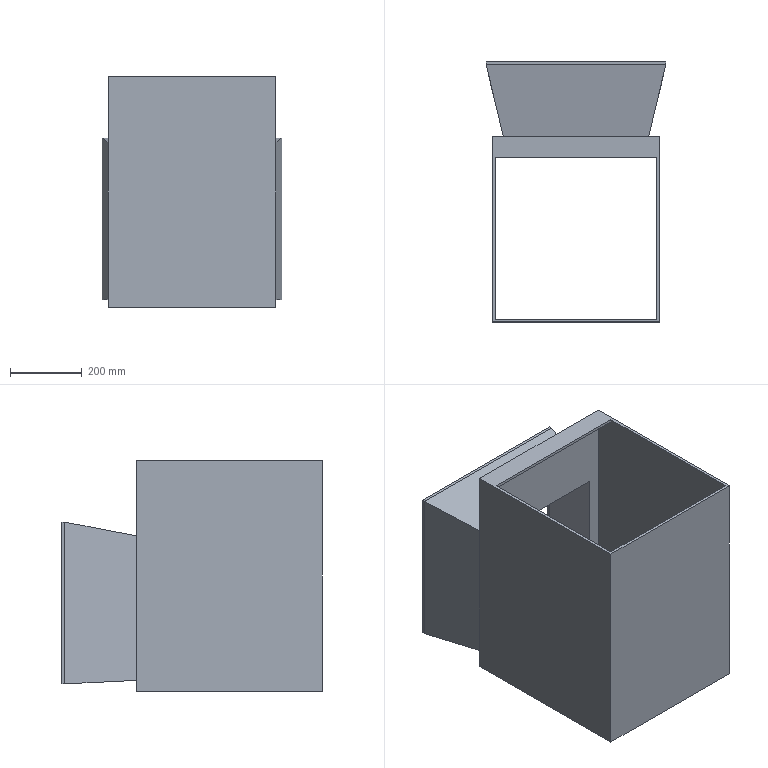Part | SolidWorks | features ICE 5, Blend 1, Extrusion 1, Shell 1 | 1 solid | 31 faces | box 500 x 724 x 640 mm | volume 11993841 mm3 | plane 31
STEP:
#1=CARTESIAN_POINT('',(191.772,250.,421.853));
#2=VERTEX_POINT('',#1);
#3=CARTESIAN_POINT('',(191.772,250.,38.009));
#4=VERTEX_POINT('',#3);
#5=CARTESIAN_POINT('',(191.772,250.,0.));
#6=DIRECTION('',(0.,0.,-1.));
#7=VECTOR('',#6,1000.);
#8=LINE('',#5,#7);
#9=EDGE_CURVE('',#2,#4,#8,.T.);
#10=ORIENTED_EDGE('',*,*,#9,.T.);
#11=CARTESIAN_POINT('',(-191.772,250.,38.009));
#12=VERTEX_POINT('',#11);
#13=CARTESIAN_POINT('',(0.,250.,38.009));
#14=DIRECTION('',(-1.,0.,0.));
#15=VECTOR('',#14,1000.);
#16=LINE('',#13,#15);
#17=EDGE_CURVE('',#4,#12,#16,.T.);
#18=ORIENTED_EDGE('',*,*,#17,.T.);
#19=CARTESIAN_POINT('',(-191.772,250.,421.853));
#20=VERTEX_POINT('',#19);
#21=CARTESIAN_POINT('',(-191.772,250.,0.));
#22=DIRECTION('',(0.,0.,1.));
#23=VECTOR('',#22,1000.);
#24=LINE('',#21,#23);
#25=EDGE_CURVE('',#12,#20,#24,.T.);
#26=ORIENTED_EDGE('',*,*,#25,.T.);
#27=CARTESIAN_POINT('',(0.,250.,421.853));
#28=DIRECTION('',(1.,0.,0.));
#29=VECTOR('',#28,1000.);
#30=LINE('',#27,#29);
#31=EDGE_CURVE('',#20,#2,#30,.T.);
#32=ORIENTED_EDGE('',*,*,#31,.T.);
#33=EDGE_LOOP('',(#10,#18,#26,#32));
#34=FACE_BOUND('',#33,.T.);
#35=CARTESIAN_POINT('',(-225.,250.,632.));
#36=VERTEX_POINT('',#35);
#37=CARTESIAN_POINT('',(225.,250.,632.));
#38=VERTEX_POINT('',#37);
#39=CARTESIAN_POINT('',(-233.,250.,632.));
#40=DIRECTION('',(1.,0.,0.));
#41=VECTOR('',#40,1000.);
#42=LINE('',#39,#41);
#43=EDGE_CURVE('',#36,#38,#42,.T.);
#44=ORIENTED_EDGE('',*,*,#43,.F.);
#45=CARTESIAN_POINT('',(-225.,250.,8.));
#46=VERTEX_POINT('',#45);
#47=CARTESIAN_POINT('',(-225.,250.,640.));
#48=DIRECTION('',(0.,0.,-1.));
#49=VECTOR('',#48,1000.);
#50=LINE('',#47,#49);
#51=EDGE_CURVE('',#36,#46,#50,.T.);
#52=ORIENTED_EDGE('',*,*,#51,.T.);
#53=CARTESIAN_POINT('',(225.,250.,8.));
#54=VERTEX_POINT('',#53);
#55=CARTESIAN_POINT('',(-233.,250.,8.));
#56=DIRECTION('',(-1.,0.,0.));
#57=VECTOR('',#56,1000.);
#58=LINE('',#55,#57);
#59=EDGE_CURVE('',#54,#46,#58,.T.);
#60=ORIENTED_EDGE('',*,*,#59,.F.);
#61=CARTESIAN_POINT('',(225.,250.,640.));
#62=DIRECTION('',(0.,0.,-1.));
#63=VECTOR('',#62,1000.);
#64=LINE('',#61,#63);
#65=EDGE_CURVE('',#38,#54,#64,.T.);
#66=ORIENTED_EDGE('',*,*,#65,.F.);
#67=EDGE_LOOP('',(#44,#52,#60,#66));
#68=FACE_OUTER_BOUND('',#67,.T.);
#69=CARTESIAN_POINT('',(0.,250.,0.));
#70=DIRECTION('',(0.,1.,0.));
#71=DIRECTION('',(0.,0.,1.));
#72=AXIS2_PLACEMENT_3D('',#69,#70,#71);
#73=PLANE('',#72);
#74=ADVANCED_FACE('',(#34,#68),#73,.F.);
#75=CARTESIAN_POINT('',(225.,200.,632.));
#76=VERTEX_POINT('',#75);
#77=CARTESIAN_POINT('',(225.,200.,640.));
#78=VERTEX_POINT('',#77);
#79=CARTESIAN_POINT('',(225.,200.,640.));
#80=DIRECTION('',(0.,0.,1.));
#81=VECTOR('',#80,1000.);
#82=LINE('',#79,#81);
#83=EDGE_CURVE('',#76,#78,#82,.T.);
#84=ORIENTED_EDGE('',*,*,#83,.F.);
#85=CARTESIAN_POINT('',(225.,250.,632.));
#86=DIRECTION('',(0.,1.,0.));
#87=VECTOR('',#86,1000.);
#88=LINE('',#85,#87);
#89=EDGE_CURVE('',#76,#38,#88,.T.);
#90=ORIENTED_EDGE('',*,*,#89,.T.);
#91=ORIENTED_EDGE('',*,*,#65,.T.);
#92=CARTESIAN_POINT('',(225.,200.,8.));
#93=VERTEX_POINT('',#92);
#94=CARTESIAN_POINT('',(225.,250.,8.));
#95=DIRECTION('',(0.,-1.,0.));
#96=VECTOR('',#95,1000.);
#97=LINE('',#94,#96);
#98=EDGE_CURVE('',#54,#93,#97,.T.);
#99=ORIENTED_EDGE('',*,*,#98,.T.);
#100=CARTESIAN_POINT('',(225.,200.,0.));
#101=VERTEX_POINT('',#100);
#102=CARTESIAN_POINT('',(225.,200.,640.));
#103=DIRECTION('',(0.,0.,-1.));
#104=VECTOR('',#103,1000.);
#105=LINE('',#102,#104);
#106=EDGE_CURVE('',#93,#101,#105,.T.);
#107=ORIENTED_EDGE('',*,*,#106,.T.);
#108=CARTESIAN_POINT('',(225.,-250.,0.));
#109=VERTEX_POINT('',#108);
#110=CARTESIAN_POINT('',(225.,250.,0.));
#111=DIRECTION('',(0.,1.,0.));
#112=VECTOR('',#111,1000.);
#113=LINE('',#110,#112);
#114=EDGE_CURVE('',#109,#101,#113,.T.);
#115=ORIENTED_EDGE('',*,*,#114,.F.);
#116=CARTESIAN_POINT('',(225.,-250.,640.));
#117=VERTEX_POINT('',#116);
#118=CARTESIAN_POINT('',(225.,-250.,640.));
#119=DIRECTION('',(0.,0.,-1.));
#120=VECTOR('',#119,1000.);
#121=LINE('',#118,#120);
#122=EDGE_CURVE('',#117,#109,#121,.T.);
#123=ORIENTED_EDGE('',*,*,#122,.F.);
#124=CARTESIAN_POINT('',(225.,250.,640.));
#125=DIRECTION('',(0.,1.,0.));
#126=VECTOR('',#125,1000.);
#127=LINE('',#124,#126);
#128=EDGE_CURVE('',#117,#78,#127,.T.);
#129=ORIENTED_EDGE('',*,*,#128,.T.);
#130=EDGE_LOOP('',(#84,#90,#91,#99,#107,#115,#123,#129));
#131=FACE_OUTER_BOUND('',#130,.T.);
#132=CARTESIAN_POINT('',(225.,250.,640.));
#133=DIRECTION('',(-1.,0.,0.));
#134=DIRECTION('',(0.,-1.,0.));
#135=AXIS2_PLACEMENT_3D('',#132,#133,#134);
#136=PLANE('',#135);
#137=ADVANCED_FACE('',(#131),#136,.T.);
#138=ORIENTED_EDGE('',*,*,#51,.F.);
#139=CARTESIAN_POINT('',(-225.,200.,632.));
#140=VERTEX_POINT('',#139);
#141=CARTESIAN_POINT('',(-225.,250.,632.));
#142=DIRECTION('',(0.,-1.,0.));
#143=VECTOR('',#142,1000.);
#144=LINE('',#141,#143);
#145=EDGE_CURVE('',#36,#140,#144,.T.);
#146=ORIENTED_EDGE('',*,*,#145,.T.);
#147=CARTESIAN_POINT('',(-225.,200.,640.));
#148=VERTEX_POINT('',#147);
#149=CARTESIAN_POINT('',(-225.,200.,640.));
#150=DIRECTION('',(0.,0.,-1.));
#151=VECTOR('',#150,1000.);
#152=LINE('',#149,#151);
#153=EDGE_CURVE('',#148,#140,#152,.T.);
#154=ORIENTED_EDGE('',*,*,#153,.F.);
#155=CARTESIAN_POINT('',(-225.,-250.,640.));
#156=VERTEX_POINT('',#155);
#157=CARTESIAN_POINT('',(-225.,250.,640.));
#158=DIRECTION('',(0.,-1.,0.));
#159=VECTOR('',#158,1000.);
#160=LINE('',#157,#159);
#161=EDGE_CURVE('',#148,#156,#160,.T.);
#162=ORIENTED_EDGE('',*,*,#161,.T.);
#163=CARTESIAN_POINT('',(-225.,-250.,0.));
#164=VERTEX_POINT('',#163);
#165=CARTESIAN_POINT('',(-225.,-250.,640.));
#166=DIRECTION('',(0.,0.,-1.));
#167=VECTOR('',#166,1000.);
#168=LINE('',#165,#167);
#169=EDGE_CURVE('',#156,#164,#168,.T.);
#170=ORIENTED_EDGE('',*,*,#169,.T.);
#171=CARTESIAN_POINT('',(-225.,200.,0.));
#172=VERTEX_POINT('',#171);
#173=CARTESIAN_POINT('',(-225.,250.,0.));
#174=DIRECTION('',(0.,-1.,0.));
#175=VECTOR('',#174,1000.);
#176=LINE('',#173,#175);
#177=EDGE_CURVE('',#172,#164,#176,.T.);
#178=ORIENTED_EDGE('',*,*,#177,.F.);
#179=CARTESIAN_POINT('',(-225.,200.,8.));
#180=VERTEX_POINT('',#179);
#181=CARTESIAN_POINT('',(-225.,200.,640.));
#182=DIRECTION('',(0.,0.,1.));
#183=VECTOR('',#182,1000.);
#184=LINE('',#181,#183);
#185=EDGE_CURVE('',#172,#180,#184,.T.);
#186=ORIENTED_EDGE('',*,*,#185,.T.);
#187=CARTESIAN_POINT('',(-225.,250.,8.));
#188=DIRECTION('',(0.,1.,0.));
#189=VECTOR('',#188,1000.);
#190=LINE('',#187,#189);
#191=EDGE_CURVE('',#180,#46,#190,.T.);
#192=ORIENTED_EDGE('',*,*,#191,.T.);
#193=EDGE_LOOP('',(#138,#146,#154,#162,#170,#178,#186,#192));
#194=FACE_OUTER_BOUND('',#193,.T.);
#195=CARTESIAN_POINT('',(-225.,250.,640.));
#196=DIRECTION('',(1.,0.,0.));
#197=DIRECTION('',(0.,1.,0.));
#198=AXIS2_PLACEMENT_3D('',#195,#196,#197);
#199=PLANE('',#198);
#200=ADVANCED_FACE('',(#194),#199,.T.);
#201=CARTESIAN_POINT('',(-250.,458.,470.));
#202=VERTEX_POINT('',#201);
#203=CARTESIAN_POINT('',(-201.923,258.,431.538));
#204=VERTEX_POINT('',#203);
#205=CARTESIAN_POINT('',(-250.,458.,470.));
#206=DIRECTION('',(0.2297,-0.9557,-0.1838));
#207=VECTOR('',#206,1000.);
#208=LINE('',#205,#207);
#209=EDGE_CURVE('',#202,#204,#208,.T.);
#210=ORIENTED_EDGE('',*,*,#209,.T.);
#211=CARTESIAN_POINT('',(201.923,258.,431.538));
#212=VERTEX_POINT('',#211);
#213=CARTESIAN_POINT('',(0.,258.,431.538));
#214=DIRECTION('',(1.,0.,0.));
#215=VECTOR('',#214,1000.);
#216=LINE('',#213,#215);
#217=EDGE_CURVE('',#204,#212,#216,.T.);
#218=ORIENTED_EDGE('',*,*,#217,.T.);
#219=CARTESIAN_POINT('',(250.,458.,470.));
#220=VERTEX_POINT('',#219);
#221=CARTESIAN_POINT('',(250.,458.,470.));
#222=DIRECTION('',(-0.2297,-0.9557,-0.1838));
#223=VECTOR('',#222,1000.);
#224=LINE('',#221,#223);
#225=EDGE_CURVE('',#220,#212,#224,.T.);
#226=ORIENTED_EDGE('',*,*,#225,.F.);
#227=CARTESIAN_POINT('',(-250.,458.,470.));
#228=DIRECTION('',(1.,0.,0.));
#229=VECTOR('',#228,1000.);
#230=LINE('',#227,#229);
#231=EDGE_CURVE('',#202,#220,#230,.T.);
#232=ORIENTED_EDGE('',*,*,#231,.F.);
#233=EDGE_LOOP('',(#210,#218,#226,#232));
#234=FACE_OUTER_BOUND('',#233,.T.);
#235=CARTESIAN_POINT('',(0.,-70.827,368.302));
#236=DIRECTION('',(0.,-0.1888,0.982));
#237=DIRECTION('',(0.,-0.982,-0.1888));
#238=AXIS2_PLACEMENT_3D('',#235,#236,#237);
#239=PLANE('',#238);
#240=ADVANCED_FACE('',(#234),#239,.T.);
#241=ORIENTED_EDGE('',*,*,#225,.T.);
#242=CARTESIAN_POINT('',(201.923,258.,29.615));
#243=VERTEX_POINT('',#242);
#244=CARTESIAN_POINT('',(201.923,258.,0.));
#245=DIRECTION('',(0.,0.,-1.));
#246=VECTOR('',#245,1000.);
#247=LINE('',#244,#246);
#248=EDGE_CURVE('',#212,#243,#247,.T.);
#249=ORIENTED_EDGE('',*,*,#248,.T.);
#250=CARTESIAN_POINT('',(250.,458.,20.));
#251=VERTEX_POINT('',#250);
#252=CARTESIAN_POINT('',(250.,458.,20.));
#253=DIRECTION('',(-0.2335,-0.9712,0.04669));
#254=VECTOR('',#253,1000.);
#255=LINE('',#252,#254);
#256=EDGE_CURVE('',#251,#243,#255,.T.);
#257=ORIENTED_EDGE('',*,*,#256,.F.);
#258=CARTESIAN_POINT('',(250.,458.,20.));
#259=DIRECTION('',(0.,0.,-1.));
#260=VECTOR('',#259,1000.);
#261=LINE('',#258,#260);
#262=EDGE_CURVE('',#220,#251,#261,.T.);
#263=ORIENTED_EDGE('',*,*,#262,.F.);
#264=EDGE_LOOP('',(#241,#249,#257,#263));
#265=FACE_OUTER_BOUND('',#264,.T.);
#266=CARTESIAN_POINT('',(132.261,-31.794,0.));
#267=DIRECTION('',(0.9723,-0.2337,0.));
#268=DIRECTION('',(0.2337,0.9723,0.));
#269=AXIS2_PLACEMENT_3D('',#266,#267,#268);
#270=PLANE('',#269);
#271=ADVANCED_FACE('',(#265),#270,.T.);
#272=ORIENTED_EDGE('',*,*,#256,.T.);
#273=CARTESIAN_POINT('',(-201.923,258.,29.615));
#274=VERTEX_POINT('',#273);
#275=CARTESIAN_POINT('',(0.,258.,29.615));
#276=DIRECTION('',(-1.,0.,0.));
#277=VECTOR('',#276,1000.);
#278=LINE('',#275,#277);
#279=EDGE_CURVE('',#243,#274,#278,.T.);
#280=ORIENTED_EDGE('',*,*,#279,.T.);
#281=CARTESIAN_POINT('',(-250.,458.,20.));
#282=VERTEX_POINT('',#281);
#283=CARTESIAN_POINT('',(-250.,458.,20.));
#284=DIRECTION('',(0.2335,-0.9712,0.04669));
#285=VECTOR('',#284,1000.);
#286=LINE('',#283,#285);
#287=EDGE_CURVE('',#282,#274,#286,.T.);
#288=ORIENTED_EDGE('',*,*,#287,.F.);
#289=CARTESIAN_POINT('',(-250.,458.,20.));
#290=DIRECTION('',(-1.,0.,0.));
#291=VECTOR('',#290,1000.);
#292=LINE('',#289,#291);
#293=EDGE_CURVE('',#251,#282,#292,.T.);
#294=ORIENTED_EDGE('',*,*,#293,.F.);
#295=EDGE_LOOP('',(#272,#280,#288,#294));
#296=FACE_OUTER_BOUND('',#295,.T.);
#297=CARTESIAN_POINT('',(0.,2.015,41.922));
#298=DIRECTION('',(0.,-0.04802,-0.9988));
#299=DIRECTION('',(0.,0.9988,-0.04802));
#300=AXIS2_PLACEMENT_3D('',#297,#298,#299);
#301=PLANE('',#300);
#302=ADVANCED_FACE('',(#296),#301,.T.);
#303=ORIENTED_EDGE('',*,*,#287,.T.);
#304=CARTESIAN_POINT('',(-201.923,258.,0.));
#305=DIRECTION('',(0.,0.,1.));
#306=VECTOR('',#305,1000.);
#307=LINE('',#304,#306);
#308=EDGE_CURVE('',#274,#204,#307,.T.);
#309=ORIENTED_EDGE('',*,*,#308,.T.);
#310=ORIENTED_EDGE('',*,*,#209,.F.);
#311=CARTESIAN_POINT('',(-250.,458.,20.));
#312=DIRECTION('',(0.,0.,1.));
#313=VECTOR('',#312,1000.);
#314=LINE('',#311,#313);
#315=EDGE_CURVE('',#282,#202,#314,.T.);
#316=ORIENTED_EDGE('',*,*,#315,.F.);
#317=EDGE_LOOP('',(#303,#309,#310,#316));
#318=FACE_OUTER_BOUND('',#317,.T.);
#319=CARTESIAN_POINT('',(-132.261,-31.794,0.));
#320=DIRECTION('',(-0.9723,-0.2337,0.));
#321=DIRECTION('',(0.2337,-0.9723,0.));
#322=AXIS2_PLACEMENT_3D('',#319,#320,#321);
#323=PLANE('',#322);
#324=ADVANCED_FACE('',(#318),#323,.T.);
#325=ORIENTED_EDGE('',*,*,#262,.T.);
#326=CARTESIAN_POINT('',(250.,466.,20.));
#327=VERTEX_POINT('',#326);
#328=CARTESIAN_POINT('',(250.,466.,20.));
#329=DIRECTION('',(0.,-1.,0.));
#330=VECTOR('',#329,1000.);
#331=LINE('',#328,#330);
#332=EDGE_CURVE('',#327,#251,#331,.T.);
#333=ORIENTED_EDGE('',*,*,#332,.F.);
#334=CARTESIAN_POINT('',(250.,466.,470.));
#335=VERTEX_POINT('',#334);
#336=CARTESIAN_POINT('',(250.,466.,20.));
#337=DIRECTION('',(0.,0.,-1.));
#338=VECTOR('',#337,1000.);
#339=LINE('',#336,#338);
#340=EDGE_CURVE('',#335,#327,#339,.T.);
#341=ORIENTED_EDGE('',*,*,#340,.F.);
#342=CARTESIAN_POINT('',(250.,466.,470.));
#343=DIRECTION('',(0.,-1.,0.));
#344=VECTOR('',#343,1000.);
#345=LINE('',#342,#344);
#346=EDGE_CURVE('',#335,#220,#345,.T.);
#347=ORIENTED_EDGE('',*,*,#346,.T.);
#348=EDGE_LOOP('',(#325,#333,#341,#347));
#349=FACE_OUTER_BOUND('',#348,.T.);
#350=CARTESIAN_POINT('',(250.,466.,20.));
#351=DIRECTION('',(-1.,0.,0.));
#352=DIRECTION('',(0.,0.,1.));
#353=AXIS2_PLACEMENT_3D('',#350,#351,#352);
#354=PLANE('',#353);
#355=ADVANCED_FACE('',(#349),#354,.F.);
#356=ORIENTED_EDGE('',*,*,#293,.T.);
#357=CARTESIAN_POINT('',(-250.,466.,20.));
#358=VERTEX_POINT('',#357);
#359=CARTESIAN_POINT('',(-250.,466.,20.));
#360=DIRECTION('',(0.,-1.,0.));
#361=VECTOR('',#360,1000.);
#362=LINE('',#359,#361);
#363=EDGE_CURVE('',#358,#282,#362,.T.);
#364=ORIENTED_EDGE('',*,*,#363,.F.);
#365=CARTESIAN_POINT('',(-250.,466.,20.));
#366=DIRECTION('',(-1.,0.,0.));
#367=VECTOR('',#366,1000.);
#368=LINE('',#365,#367);
#369=EDGE_CURVE('',#327,#358,#368,.T.);
#370=ORIENTED_EDGE('',*,*,#369,.F.);
#371=ORIENTED_EDGE('',*,*,#332,.T.);
#372=EDGE_LOOP('',(#356,#364,#370,#371));
#373=FACE_OUTER_BOUND('',#372,.T.);
#374=CARTESIAN_POINT('',(-250.,466.,20.));
#375=DIRECTION('',(0.,0.,1.));
#376=DIRECTION('',(1.,0.,0.));
#377=AXIS2_PLACEMENT_3D('',#374,#375,#376);
#378=PLANE('',#377);
#379=ADVANCED_FACE('',(#373),#378,.F.);
#380=ORIENTED_EDGE('',*,*,#315,.T.);
#381=CARTESIAN_POINT('',(-250.,466.,470.));
#382=VERTEX_POINT('',#381);
#383=CARTESIAN_POINT('',(-250.,466.,470.));
#384=DIRECTION('',(0.,-1.,0.));
#385=VECTOR('',#384,1000.);
#386=LINE('',#383,#385);
#387=EDGE_CURVE('',#382,#202,#386,.T.);
#388=ORIENTED_EDGE('',*,*,#387,.F.);
#389=CARTESIAN_POINT('',(-250.,466.,20.));
#390=DIRECTION('',(0.,0.,1.));
#391=VECTOR('',#390,1000.);
#392=LINE('',#389,#391);
#393=EDGE_CURVE('',#358,#382,#392,.T.);
#394=ORIENTED_EDGE('',*,*,#393,.F.);
#395=ORIENTED_EDGE('',*,*,#363,.T.);
#396=EDGE_LOOP('',(#380,#388,#394,#395));
#397=FACE_OUTER_BOUND('',#396,.T.);
#398=CARTESIAN_POINT('',(-250.,466.,20.));
#399=DIRECTION('',(1.,0.,0.));
#400=DIRECTION('',(0.,0.,-1.));
#401=AXIS2_PLACEMENT_3D('',#398,#399,#400);
#402=PLANE('',#401);
#403=ADVANCED_FACE('',(#397),#402,.F.);
#404=ORIENTED_EDGE('',*,*,#231,.T.);
#405=ORIENTED_EDGE('',*,*,#346,.F.);
#406=CARTESIAN_POINT('',(-250.,466.,470.));
#407=DIRECTION('',(1.,0.,0.));
#408=VECTOR('',#407,1000.);
#409=LINE('',#406,#408);
#410=EDGE_CURVE('',#382,#335,#409,.T.);
#411=ORIENTED_EDGE('',*,*,#410,.F.);
#412=ORIENTED_EDGE('',*,*,#387,.T.);
#413=EDGE_LOOP('',(#404,#405,#411,#412));
#414=FACE_OUTER_BOUND('',#413,.T.);
#415=CARTESIAN_POINT('',(-250.,466.,470.));
#416=DIRECTION('',(0.,0.,-1.));
#417=DIRECTION('',(-1.,0.,0.));
#418=AXIS2_PLACEMENT_3D('',#415,#416,#417);
#419=PLANE('',#418);
#420=ADVANCED_FACE('',(#414),#419,.F.);
#421=CARTESIAN_POINT('',(242.,466.,462.));
#422=VERTEX_POINT('',#421);
#423=CARTESIAN_POINT('',(242.,466.,28.));
#424=VERTEX_POINT('',#423);
#425=CARTESIAN_POINT('',(242.,466.,20.));
#426=DIRECTION('',(0.,0.,-1.));
#427=VECTOR('',#426,1000.);
#428=LINE('',#425,#427);
#429=EDGE_CURVE('',#422,#424,#428,.T.);
#430=ORIENTED_EDGE('',*,*,#429,.F.);
#431=CARTESIAN_POINT('',(-242.,466.,462.));
#432=VERTEX_POINT('',#431);
#433=CARTESIAN_POINT('',(-250.,466.,462.));
#434=DIRECTION('',(1.,0.,0.));
#435=VECTOR('',#434,1000.);
#436=LINE('',#433,#435);
#437=EDGE_CURVE('',#432,#422,#436,.T.);
#438=ORIENTED_EDGE('',*,*,#437,.F.);
#439=CARTESIAN_POINT('',(-242.,466.,28.));
#440=VERTEX_POINT('',#439);
#441=CARTESIAN_POINT('',(-242.,466.,20.));
#442=DIRECTION('',(0.,0.,1.));
#443=VECTOR('',#442,1000.);
#444=LINE('',#441,#443);
#445=EDGE_CURVE('',#440,#432,#444,.T.);
#446=ORIENTED_EDGE('',*,*,#445,.F.);
#447=CARTESIAN_POINT('',(-250.,466.,28.));
#448=DIRECTION('',(-1.,0.,0.));
#449=VECTOR('',#448,1000.);
#450=LINE('',#447,#449);
#451=EDGE_CURVE('',#424,#440,#450,.T.);
#452=ORIENTED_EDGE('',*,*,#451,.F.);
#453=EDGE_LOOP('',(#430,#438,#446,#452));
#454=FACE_BOUND('',#453,.T.);
#455=ORIENTED_EDGE('',*,*,#340,.T.);
#456=ORIENTED_EDGE('',*,*,#369,.T.);
#457=ORIENTED_EDGE('',*,*,#393,.T.);
#458=ORIENTED_EDGE('',*,*,#410,.T.);
#459=EDGE_LOOP('',(#455,#456,#457,#458));
#460=FACE_OUTER_BOUND('',#459,.T.);
#461=CARTESIAN_POINT('',(0.,466.,0.));
#462=DIRECTION('',(0.,1.,0.));
#463=DIRECTION('',(0.,0.,1.));
#464=AXIS2_PLACEMENT_3D('',#461,#462,#463);
#465=PLANE('',#464);
#466=ADVANCED_FACE('',(#454,#460),#465,.T.);
#467=ORIENTED_EDGE('',*,*,#161,.F.);
#468=CARTESIAN_POINT('',(-233.,200.,640.));
#469=DIRECTION('',(-1.,0.,0.));
#470=VECTOR('',#469,1000.);
#471=LINE('',#468,#470);
#472=EDGE_CURVE('',#78,#148,#471,.T.);
#473=ORIENTED_EDGE('',*,*,#472,.F.);
#474=ORIENTED_EDGE('',*,*,#128,.F.);
#475=CARTESIAN_POINT('',(-225.,-250.,640.));
#476=DIRECTION('',(1.,0.,0.));
#477=VECTOR('',#476,1000.);
#478=LINE('',#475,#477);
#479=EDGE_CURVE('',#156,#117,#478,.T.);
#480=ORIENTED_EDGE('',*,*,#479,.F.);
#481=EDGE_LOOP('',(#467,#473,#474,#480));
#482=FACE_BOUND('',#481,.T.);
#483=CARTESIAN_POINT('',(-233.,258.,640.));
#484=VERTEX_POINT('',#483);
#485=CARTESIAN_POINT('',(-233.,-258.,640.));
#486=VERTEX_POINT('',#485);
#487=CARTESIAN_POINT('',(-233.,258.,640.));
#488=DIRECTION('',(0.,-1.,0.));
#489=VECTOR('',#488,1000.);
#490=LINE('',#487,#489);
#491=EDGE_CURVE('',#484,#486,#490,.T.);
#492=ORIENTED_EDGE('',*,*,#491,.T.);
#493=CARTESIAN_POINT('',(233.,-258.,640.));
#494=VERTEX_POINT('',#493);
#495=CARTESIAN_POINT('',(-233.,-258.,640.));
#496=DIRECTION('',(1.,0.,0.));
#497=VECTOR('',#496,1000.);
#498=LINE('',#495,#497);
#499=EDGE_CURVE('',#486,#494,#498,.T.);
#500=ORIENTED_EDGE('',*,*,#499,.T.);
#501=CARTESIAN_POINT('',(233.,258.,640.));
#502=VERTEX_POINT('',#501);
#503=CARTESIAN_POINT('',(233.,258.,640.));
#504=DIRECTION('',(0.,1.,0.));
#505=VECTOR('',#504,1000.);
#506=LINE('',#503,#505);
#507=EDGE_CURVE('',#494,#502,#506,.T.);
#508=ORIENTED_EDGE('',*,*,#507,.T.);
#509=CARTESIAN_POINT('',(-233.,258.,640.));
#510=DIRECTION('',(-1.,0.,0.));
#511=VECTOR('',#510,1000.);
#512=LINE('',#509,#511);
#513=EDGE_CURVE('',#502,#484,#512,.T.);
#514=ORIENTED_EDGE('',*,*,#513,.T.);
#515=EDGE_LOOP('',(#492,#500,#508,#514));
#516=FACE_OUTER_BOUND('',#515,.T.);
#517=CARTESIAN_POINT('',(0.,0.,640.));
#518=DIRECTION('',(0.,0.,1.));
#519=DIRECTION('',(1.,0.,0.));
#520=AXIS2_PLACEMENT_3D('',#517,#518,#519);
#521=PLANE('',#520);
#522=ADVANCED_FACE('',(#482,#516),#521,.T.);
#523=ORIENTED_EDGE('',*,*,#114,.T.);
#524=CARTESIAN_POINT('',(-233.,200.,0.));
#525=DIRECTION('',(1.,0.,0.));
#526=VECTOR('',#525,1000.);
#527=LINE('',#524,#526);
#528=EDGE_CURVE('',#172,#101,#527,.T.);
#529=ORIENTED_EDGE('',*,*,#528,.F.);
#530=ORIENTED_EDGE('',*,*,#177,.T.);
#531=CARTESIAN_POINT('',(-225.,-250.,0.));
#532=DIRECTION('',(1.,0.,0.));
#533=VECTOR('',#532,1000.);
#534=LINE('',#531,#533);
#535=EDGE_CURVE('',#164,#109,#534,.T.);
#536=ORIENTED_EDGE('',*,*,#535,.T.);
#537=EDGE_LOOP('',(#523,#529,#530,#536));
#538=FACE_BOUND('',#537,.T.);
#539=CARTESIAN_POINT('',(233.,258.,0.));
#540=VERTEX_POINT('',#539);
#541=CARTESIAN_POINT('',(-233.,258.,0.));
#542=VERTEX_POINT('',#541);
#543=CARTESIAN_POINT('',(-233.,258.,0.));
#544=DIRECTION('',(-1.,0.,0.));
#545=VECTOR('',#544,1000.);
#546=LINE('',#543,#545);
#547=EDGE_CURVE('',#540,#542,#546,.T.);
#548=ORIENTED_EDGE('',*,*,#547,.F.);
#549=CARTESIAN_POINT('',(233.,-258.,0.));
#550=VERTEX_POINT('',#549);
#551=CARTESIAN_POINT('',(233.,258.,0.));
#552=DIRECTION('',(0.,1.,0.));
#553=VECTOR('',#552,1000.);
#554=LINE('',#551,#553);
#555=EDGE_CURVE('',#550,#540,#554,.T.);
#556=ORIENTED_EDGE('',*,*,#555,.F.);
#557=CARTESIAN_POINT('',(-233.,-258.,0.));
#558=VERTEX_POINT('',#557);
#559=CARTESIAN_POINT('',(-233.,-258.,0.));
#560=DIRECTION('',(1.,0.,0.));
#561=VECTOR('',#560,1000.);
#562=LINE('',#559,#561);
#563=EDGE_CURVE('',#558,#550,#562,.T.);
#564=ORIENTED_EDGE('',*,*,#563,.F.);
#565=CARTESIAN_POINT('',(-233.,258.,0.));
#566=DIRECTION('',(0.,-1.,0.));
#567=VECTOR('',#566,1000.);
#568=LINE('',#565,#567);
#569=EDGE_CURVE('',#542,#558,#568,.T.);
#570=ORIENTED_EDGE('',*,*,#569,.F.);
#571=EDGE_LOOP('',(#548,#556,#564,#570));
#572=FACE_OUTER_BOUND('',#571,.T.);
#573=CARTESIAN_POINT('',(0.,0.,0.));
#574=DIRECTION('',(0.,0.,1.));
#575=DIRECTION('',(1.,0.,0.));
#576=AXIS2_PLACEMENT_3D('',#573,#574,#575);
#577=PLANE('',#576);
#578=ADVANCED_FACE('',(#538,#572),#577,.F.);
#579=CARTESIAN_POINT('',(233.,258.,640.));
#580=DIRECTION('',(0.,0.,-1.));
#581=VECTOR('',#580,1000.);
#582=LINE('',#579,#581);
#583=EDGE_CURVE('',#502,#540,#582,.T.);
#584=ORIENTED_EDGE('',*,*,#583,.F.);
#585=ORIENTED_EDGE('',*,*,#507,.F.);
#586=CARTESIAN_POINT('',(233.,-258.,640.));
#587=DIRECTION('',(0.,0.,-1.));
#588=VECTOR('',#587,1000.);
#589=LINE('',#586,#588);
#590=EDGE_CURVE('',#494,#550,#589,.T.);
#591=ORIENTED_EDGE('',*,*,#590,.T.);
#592=ORIENTED_EDGE('',*,*,#555,.T.);
#593=EDGE_LOOP('',(#584,#585,#591,#592));
#594=FACE_OUTER_BOUND('',#593,.T.);
#595=CARTESIAN_POINT('',(233.,258.,640.));
#596=DIRECTION('',(-1.,0.,0.));
#597=DIRECTION('',(0.,-1.,0.));
#598=AXIS2_PLACEMENT_3D('',#595,#596,#597);
#599=PLANE('',#598);
#600=ADVANCED_FACE('',(#594),#599,.F.);
#601=ORIENTED_EDGE('',*,*,#217,.F.);
#602=ORIENTED_EDGE('',*,*,#308,.F.);
#603=ORIENTED_EDGE('',*,*,#279,.F.);
#604=ORIENTED_EDGE('',*,*,#248,.F.);
#605=EDGE_LOOP('',(#601,#602,#603,#604));
#606=FACE_BOUND('',#605,.T.);
#607=ORIENTED_EDGE('',*,*,#547,.T.);
#608=CARTESIAN_POINT('',(-233.,258.,640.));
#609=DIRECTION('',(0.,0.,-1.));
#610=VECTOR('',#609,1000.);
#611=LINE('',#608,#610);
#612=EDGE_CURVE('',#484,#542,#611,.T.);
#613=ORIENTED_EDGE('',*,*,#612,.F.);
#614=ORIENTED_EDGE('',*,*,#513,.F.);
#615=ORIENTED_EDGE('',*,*,#583,.T.);
#616=EDGE_LOOP('',(#607,#613,#614,#615));
#617=FACE_OUTER_BOUND('',#616,.T.);
#618=CARTESIAN_POINT('',(-233.,258.,640.));
#619=DIRECTION('',(0.,-1.,0.));
#620=DIRECTION('',(0.,0.,-1.));
#621=AXIS2_PLACEMENT_3D('',#618,#619,#620);
#622=PLANE('',#621);
#623=ADVANCED_FACE('',(#606,#617),#622,.F.);
#624=ORIENTED_EDGE('',*,*,#569,.T.);
#625=CARTESIAN_POINT('',(-233.,-258.,640.));
#626=DIRECTION('',(0.,0.,-1.));
#627=VECTOR('',#626,1000.);
#628=LINE('',#625,#627);
#629=EDGE_CURVE('',#486,#558,#628,.T.);
#630=ORIENTED_EDGE('',*,*,#629,.F.);
#631=ORIENTED_EDGE('',*,*,#491,.F.);
#632=ORIENTED_EDGE('',*,*,#612,.T.);
#633=EDGE_LOOP('',(#624,#630,#631,#632));
#634=FACE_OUTER_BOUND('',#633,.T.);
#635=CARTESIAN_POINT('',(-233.,258.,640.));
#636=DIRECTION('',(1.,0.,0.));
#637=DIRECTION('',(0.,1.,0.));
#638=AXIS2_PLACEMENT_3D('',#635,#636,#637);
#639=PLANE('',#638);
#640=ADVANCED_FACE('',(#634),#639,.F.);
#641=ORIENTED_EDGE('',*,*,#563,.T.);
#642=ORIENTED_EDGE('',*,*,#590,.F.);
#643=ORIENTED_EDGE('',*,*,#499,.F.);
#644=ORIENTED_EDGE('',*,*,#629,.T.);
#645=EDGE_LOOP('',(#641,#642,#643,#644));
#646=FACE_OUTER_BOUND('',#645,.T.);
#647=CARTESIAN_POINT('',(-233.,-258.,640.));
#648=DIRECTION('',(0.,1.,0.));
#649=DIRECTION('',(0.,0.,1.));
#650=AXIS2_PLACEMENT_3D('',#647,#648,#649);
#651=PLANE('',#650);
#652=ADVANCED_FACE('',(#646),#651,.F.);
#653=ORIENTED_EDGE('',*,*,#535,.F.);
#654=ORIENTED_EDGE('',*,*,#169,.F.);
#655=ORIENTED_EDGE('',*,*,#479,.T.);
#656=ORIENTED_EDGE('',*,*,#122,.T.);
#657=EDGE_LOOP('',(#653,#654,#655,#656));
#658=FACE_OUTER_BOUND('',#657,.T.);
#659=CARTESIAN_POINT('',(-225.,-250.,640.));
#660=DIRECTION('',(0.,1.,0.));
#661=DIRECTION('',(0.,0.,1.));
#662=AXIS2_PLACEMENT_3D('',#659,#660,#661);
#663=PLANE('',#662);
#664=ADVANCED_FACE('',(#658),#663,.T.);
#665=CARTESIAN_POINT('',(241.955,458.762,462.));
#666=VERTEX_POINT('',#665);
#667=CARTESIAN_POINT('',(108.943,-94.571,355.59));
#668=DIRECTION('',(-0.2297,-0.9557,-0.1838));
#669=VECTOR('',#668,1000.);
#670=LINE('',#667,#669);
#671=EDGE_CURVE('',#666,#2,#670,.T.);
#672=ORIENTED_EDGE('',*,*,#671,.F.);
#673=CARTESIAN_POINT('',(242.,458.948,462.));
#674=VERTEX_POINT('',#673);
#675=CARTESIAN_POINT('',(124.483,-29.924,462.));
#676=DIRECTION('',(0.2337,0.9723,0.));
#677=VECTOR('',#676,1000.);
#678=LINE('',#675,#677);
#679=EDGE_CURVE('',#666,#674,#678,.T.);
#680=ORIENTED_EDGE('',*,*,#679,.T.);
#681=CARTESIAN_POINT('',(242.,458.948,28.));
#682=VERTEX_POINT('',#681);
#683=CARTESIAN_POINT('',(242.,458.948,0.));
#684=DIRECTION('',(0.,0.,-1.));
#685=VECTOR('',#684,1000.);
#686=LINE('',#683,#685);
#687=EDGE_CURVE('',#674,#682,#686,.T.);
#688=ORIENTED_EDGE('',*,*,#687,.T.);
#689=CARTESIAN_POINT('',(241.818,458.192,28.));
#690=VERTEX_POINT('',#689);
#691=CARTESIAN_POINT('',(216.726,353.806,28.));
#692=DIRECTION('',(0.2337,0.9723,0.));
#693=VECTOR('',#692,1000.);
#694=LINE('',#691,#693);
#695=EDGE_CURVE('',#690,#682,#694,.T.);
#696=ORIENTED_EDGE('',*,*,#695,.F.);
#697=CARTESIAN_POINT('',(125.044,-27.59,51.355));
#698=DIRECTION('',(-0.2335,-0.9712,0.04669));
#699=VECTOR('',#698,1000.);
#700=LINE('',#697,#699);
#701=EDGE_CURVE('',#690,#4,#700,.T.);
#702=ORIENTED_EDGE('',*,*,#701,.T.);
#703=ORIENTED_EDGE('',*,*,#9,.F.);
#704=EDGE_LOOP('',(#672,#680,#688,#696,#702,#703));
#705=FACE_OUTER_BOUND('',#704,.T.);
#706=CARTESIAN_POINT('',(124.483,-29.924,0.));
#707=DIRECTION('',(0.9723,-0.2337,0.));
#708=DIRECTION('',(0.2337,0.9723,0.));
#709=AXIS2_PLACEMENT_3D('',#706,#707,#708);
#710=PLANE('',#709);
#711=ADVANCED_FACE('',(#705),#710,.F.);
#712=ORIENTED_EDGE('',*,*,#701,.F.);
#713=CARTESIAN_POINT('',(-241.818,458.192,28.));
#714=VERTEX_POINT('',#713);
#715=CARTESIAN_POINT('',(0.,458.192,28.));
#716=DIRECTION('',(-1.,0.,0.));
#717=VECTOR('',#716,1000.);
#718=LINE('',#715,#717);
#719=EDGE_CURVE('',#690,#714,#718,.T.);
#720=ORIENTED_EDGE('',*,*,#719,.T.);
#721=CARTESIAN_POINT('',(-125.044,-27.59,51.355));
#722=DIRECTION('',(0.2335,-0.9712,0.04669));
#723=VECTOR('',#722,1000.);
#724=LINE('',#721,#723);
#725=EDGE_CURVE('',#714,#12,#724,.T.);
#726=ORIENTED_EDGE('',*,*,#725,.T.);
#727=ORIENTED_EDGE('',*,*,#17,.F.);
#728=EDGE_LOOP('',(#712,#720,#726,#727));
#729=FACE_OUTER_BOUND('',#728,.T.);
#730=CARTESIAN_POINT('',(0.,2.4,49.913));
#731=DIRECTION('',(0.,-0.04802,-0.9988));
#732=DIRECTION('',(0.,0.9988,-0.04802));
#733=AXIS2_PLACEMENT_3D('',#730,#731,#732);
#734=PLANE('',#733);
#735=ADVANCED_FACE('',(#729),#734,.F.);
#736=CARTESIAN_POINT('',(-241.955,458.762,462.));
#737=VERTEX_POINT('',#736);
#738=CARTESIAN_POINT('',(-108.943,-94.571,355.59));
#739=DIRECTION('',(0.2297,-0.9557,-0.1838));
#740=VECTOR('',#739,1000.);
#741=LINE('',#738,#740);
#742=EDGE_CURVE('',#737,#20,#741,.T.);
#743=ORIENTED_EDGE('',*,*,#742,.F.);
#744=CARTESIAN_POINT('',(0.,458.762,462.));
#745=DIRECTION('',(1.,0.,0.));
#746=VECTOR('',#745,1000.);
#747=LINE('',#744,#746);
#748=EDGE_CURVE('',#737,#666,#747,.T.);
#749=ORIENTED_EDGE('',*,*,#748,.T.);
#750=ORIENTED_EDGE('',*,*,#671,.T.);
#751=ORIENTED_EDGE('',*,*,#31,.F.);
#752=EDGE_LOOP('',(#743,#749,#750,#751));
#753=FACE_OUTER_BOUND('',#752,.T.);
#754=CARTESIAN_POINT('',(0.,-69.317,360.446));
#755=DIRECTION('',(0.,-0.1888,0.982));
#756=DIRECTION('',(0.,-0.982,-0.1888));
#757=AXIS2_PLACEMENT_3D('',#754,#755,#756);
#758=PLANE('',#757);
#759=ADVANCED_FACE('',(#753),#758,.F.);
#760=ORIENTED_EDGE('',*,*,#725,.F.);
#761=CARTESIAN_POINT('',(-242.,458.948,28.));
#762=VERTEX_POINT('',#761);
#763=CARTESIAN_POINT('',(-124.483,-29.924,28.));
#764=DIRECTION('',(-0.2337,0.9723,0.));
#765=VECTOR('',#764,1000.);
#766=LINE('',#763,#765);
#767=EDGE_CURVE('',#714,#762,#766,.T.);
#768=ORIENTED_EDGE('',*,*,#767,.T.);
#769=CARTESIAN_POINT('',(-242.,458.948,462.));
#770=VERTEX_POINT('',#769);
#771=CARTESIAN_POINT('',(-242.,458.948,0.));
#772=DIRECTION('',(0.,0.,1.));
#773=VECTOR('',#772,1000.);
#774=LINE('',#771,#773);
#775=EDGE_CURVE('',#762,#770,#774,.T.);
#776=ORIENTED_EDGE('',*,*,#775,.T.);
#777=CARTESIAN_POINT('',(-244.04,467.433,462.));
#778=DIRECTION('',(-0.2337,0.9723,0.));
#779=VECTOR('',#778,1000.);
#780=LINE('',#777,#779);
#781=EDGE_CURVE('',#737,#770,#780,.T.);
#782=ORIENTED_EDGE('',*,*,#781,.F.);
#783=ORIENTED_EDGE('',*,*,#742,.T.);
#784=ORIENTED_EDGE('',*,*,#25,.F.);
#785=EDGE_LOOP('',(#760,#768,#776,#782,#783,#784));
#786=FACE_OUTER_BOUND('',#785,.T.);
#787=CARTESIAN_POINT('',(-124.483,-29.924,0.));
#788=DIRECTION('',(-0.9723,-0.2337,0.));
#789=DIRECTION('',(0.2337,-0.9723,0.));
#790=AXIS2_PLACEMENT_3D('',#787,#788,#789);
#791=PLANE('',#790);
#792=ADVANCED_FACE('',(#786),#791,.F.);
#793=ORIENTED_EDGE('',*,*,#687,.F.);
#794=CARTESIAN_POINT('',(242.,466.,462.));
#795=DIRECTION('',(0.,-1.,0.));
#796=VECTOR('',#795,1000.);
#797=LINE('',#794,#796);
#798=EDGE_CURVE('',#422,#674,#797,.T.);
#799=ORIENTED_EDGE('',*,*,#798,.F.);
#800=ORIENTED_EDGE('',*,*,#429,.T.);
#801=CARTESIAN_POINT('',(242.,466.,28.));
#802=DIRECTION('',(0.,-1.,0.));
#803=VECTOR('',#802,1000.);
#804=LINE('',#801,#803);
#805=EDGE_CURVE('',#424,#682,#804,.T.);
#806=ORIENTED_EDGE('',*,*,#805,.T.);
#807=EDGE_LOOP('',(#793,#799,#800,#806));
#808=FACE_OUTER_BOUND('',#807,.T.);
#809=CARTESIAN_POINT('',(242.,466.,20.));
#810=DIRECTION('',(-1.,0.,0.));
#811=DIRECTION('',(0.,0.,1.));
#812=AXIS2_PLACEMENT_3D('',#809,#810,#811);
#813=PLANE('',#812);
#814=ADVANCED_FACE('',(#808),#813,.T.);
#815=ORIENTED_EDGE('',*,*,#719,.F.);
#816=ORIENTED_EDGE('',*,*,#695,.T.);
#817=ORIENTED_EDGE('',*,*,#805,.F.);
#818=ORIENTED_EDGE('',*,*,#451,.T.);
#819=CARTESIAN_POINT('',(-242.,466.,28.));
#820=DIRECTION('',(0.,-1.,0.));
#821=VECTOR('',#820,1000.);
#822=LINE('',#819,#821);
#823=EDGE_CURVE('',#440,#762,#822,.T.);
#824=ORIENTED_EDGE('',*,*,#823,.T.);
#825=ORIENTED_EDGE('',*,*,#767,.F.);
#826=EDGE_LOOP('',(#815,#816,#817,#818,#824,#825));
#827=FACE_OUTER_BOUND('',#826,.T.);
#828=CARTESIAN_POINT('',(-250.,466.,28.));
#829=DIRECTION('',(0.,0.,1.));
#830=DIRECTION('',(1.,0.,0.));
#831=AXIS2_PLACEMENT_3D('',#828,#829,#830);
#832=PLANE('',#831);
#833=ADVANCED_FACE('',(#827),#832,.T.);
#834=ORIENTED_EDGE('',*,*,#775,.F.);
#835=ORIENTED_EDGE('',*,*,#823,.F.);
#836=ORIENTED_EDGE('',*,*,#445,.T.);
#837=CARTESIAN_POINT('',(-242.,466.,462.));
#838=DIRECTION('',(0.,-1.,0.));
#839=VECTOR('',#838,1000.);
#840=LINE('',#837,#839);
#841=EDGE_CURVE('',#432,#770,#840,.T.);
#842=ORIENTED_EDGE('',*,*,#841,.T.);
#843=EDGE_LOOP('',(#834,#835,#836,#842));
#844=FACE_OUTER_BOUND('',#843,.T.);
#845=CARTESIAN_POINT('',(-242.,466.,20.));
#846=DIRECTION('',(1.,0.,0.));
#847=DIRECTION('',(0.,0.,-1.));
#848=AXIS2_PLACEMENT_3D('',#845,#846,#847);
#849=PLANE('',#848);
#850=ADVANCED_FACE('',(#844),#849,.T.);
#851=ORIENTED_EDGE('',*,*,#748,.F.);
#852=ORIENTED_EDGE('',*,*,#781,.T.);
#853=ORIENTED_EDGE('',*,*,#841,.F.);
#854=ORIENTED_EDGE('',*,*,#437,.T.);
#855=ORIENTED_EDGE('',*,*,#798,.T.);
#856=ORIENTED_EDGE('',*,*,#679,.F.);
#857=EDGE_LOOP('',(#851,#852,#853,#854,#855,#856));
#858=FACE_OUTER_BOUND('',#857,.T.);
#859=CARTESIAN_POINT('',(-250.,466.,462.));
#860=DIRECTION('',(0.,0.,-1.));
#861=DIRECTION('',(-1.,0.,0.));
#862=AXIS2_PLACEMENT_3D('',#859,#860,#861);
#863=PLANE('',#862);
#864=ADVANCED_FACE('',(#858),#863,.T.);
#865=ORIENTED_EDGE('',*,*,#98,.F.);
#866=ORIENTED_EDGE('',*,*,#59,.T.);
#867=ORIENTED_EDGE('',*,*,#191,.F.);
#868=CARTESIAN_POINT('',(-233.,200.,8.));
#869=DIRECTION('',(-1.,0.,0.));
#870=VECTOR('',#869,1000.);
#871=LINE('',#868,#870);
#872=EDGE_CURVE('',#93,#180,#871,.T.);
#873=ORIENTED_EDGE('',*,*,#872,.F.);
#874=EDGE_LOOP('',(#865,#866,#867,#873));
#875=FACE_OUTER_BOUND('',#874,.T.);
#876=CARTESIAN_POINT('',(-233.,200.,8.));
#877=DIRECTION('',(0.,0.,-1.));
#878=DIRECTION('',(-1.,0.,0.));
#879=AXIS2_PLACEMENT_3D('',#876,#877,#878);
#880=PLANE('',#879);
#881=ADVANCED_FACE('',(#875),#880,.F.);
#882=ORIENTED_EDGE('',*,*,#106,.F.);
#883=ORIENTED_EDGE('',*,*,#872,.T.);
#884=ORIENTED_EDGE('',*,*,#185,.F.);
#885=ORIENTED_EDGE('',*,*,#528,.T.);
#886=EDGE_LOOP('',(#882,#883,#884,#885));
#887=FACE_OUTER_BOUND('',#886,.T.);
#888=CARTESIAN_POINT('',(0.,200.,0.));
#889=DIRECTION('',(0.,1.,0.));
#890=DIRECTION('',(0.,0.,1.));
#891=AXIS2_PLACEMENT_3D('',#888,#889,#890);
#892=PLANE('',#891);
#893=ADVANCED_FACE('',(#887),#892,.F.);
#894=ORIENTED_EDGE('',*,*,#89,.F.);
#895=CARTESIAN_POINT('',(-233.,200.,632.));
#896=DIRECTION('',(1.,0.,0.));
#897=VECTOR('',#896,1000.);
#898=LINE('',#895,#897);
#899=EDGE_CURVE('',#140,#76,#898,.T.);
#900=ORIENTED_EDGE('',*,*,#899,.F.);
#901=ORIENTED_EDGE('',*,*,#145,.F.);
#902=ORIENTED_EDGE('',*,*,#43,.T.);
#903=EDGE_LOOP('',(#894,#900,#901,#902));
#904=FACE_OUTER_BOUND('',#903,.T.);
#905=CARTESIAN_POINT('',(-233.,200.,632.));
#906=DIRECTION('',(0.,0.,1.));
#907=DIRECTION('',(1.,0.,0.));
#908=AXIS2_PLACEMENT_3D('',#905,#906,#907);
#909=PLANE('',#908);
#910=ADVANCED_FACE('',(#904),#909,.F.);
#911=ORIENTED_EDGE('',*,*,#899,.T.);
#912=ORIENTED_EDGE('',*,*,#83,.T.);
#913=ORIENTED_EDGE('',*,*,#472,.T.);
#914=ORIENTED_EDGE('',*,*,#153,.T.);
#915=EDGE_LOOP('',(#911,#912,#913,#914));
#916=FACE_OUTER_BOUND('',#915,.T.);
#917=CARTESIAN_POINT('',(0.,200.,0.));
#918=DIRECTION('',(0.,-1.,0.));
#919=DIRECTION('',(0.,0.,-1.));
#920=AXIS2_PLACEMENT_3D('',#917,#918,#919);
#921=PLANE('',#920);
#922=ADVANCED_FACE('',(#916),#921,.T.);
#923=CLOSED_SHELL('',(#74,#137,#200,#240,#271,#302,#324,#355,#379,#403,#420,#466,#522,#578,#600,#623,#640,#652,#664,#711,#735,#759,#792,#814,#833,#850,#864,#881,#893,#910,#922));
#924=MANIFOLD_SOLID_BREP('',#923);
#925=CARTESIAN_POINT('',(0.,0.,0.));
#926=DIRECTION('',(0.,0.,1.));
#927=DIRECTION('',(1.,0.,0.));
#928=AXIS2_PLACEMENT_3D('',#925,#926,#927);
#929=(LENGTH_UNIT()NAMED_UNIT(*)SI_UNIT(.MILLI.,.METRE.));
#930=UNCERTAINTY_MEASURE_WITH_UNIT(LENGTH_MEASURE(0.00001),#929,'','');
#931=(NAMED_UNIT(*)PLANE_ANGLE_UNIT()SI_UNIT($,.RADIAN.));
#932=(NAMED_UNIT(*)SI_UNIT($,.STERADIAN.)SOLID_ANGLE_UNIT());
#933=(GEOMETRIC_REPRESENTATION_CONTEXT(3)GLOBAL_UNCERTAINTY_ASSIGNED_CONTEXT((#930))GLOBAL_UNIT_ASSIGNED_CONTEXT((#929,#931,#932))REPRESENTATION_CONTEXT('',''));
#934=ADVANCED_BREP_SHAPE_REPRESENTATION('',(#924,#928),#933);